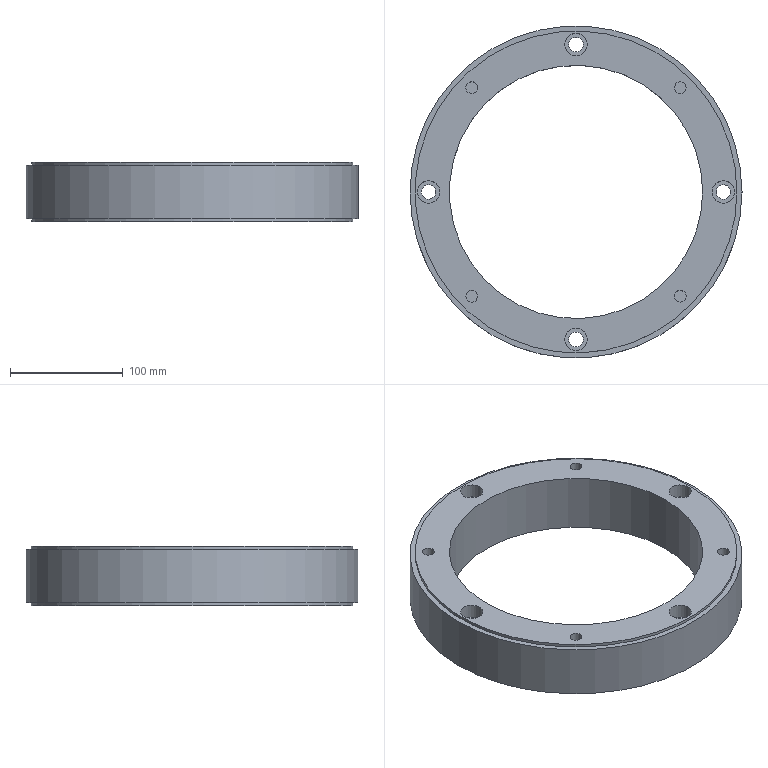CAM job | NX | 3-axis milling, drilling | part box 295 x 295 x 53 mm | stock box 301 x 301 x 54 mm
Tools:
number,name,description,diameter,corner_radius,flute_length,length,flutes
1,D63,Milling Tool-5 Parameters,63.0,0.0,50.0,75.0,2
7,D6A45,Milling Tool-5 Parameters,6.0,0.0,3.0,3.0,2
14,10.5ZT,Drilling Tool,10.5,0.0,35.0,50.0,2
13,13.0ZT,Drilling Tool,13.0,0.0,35.0,50.0,2
11,D10JING,Milling Tool-5 Parameters,10.0,0.0,50.0,75.0,2
17,D17R0.8,Milling Tool-5 Parameters,17.0,0.0,50.0,75.0,2
Operations:
program,operation,operation_type,tool,method,geometry_group,spindle_rpm,surface_speed,feed_per_tooth,feed_cut,feed_plunge,cut_length_mm,path_length_mm,cut_time_min,machine_time_min
1,FLOOR_WALL,VolumeBased25DMillingOperation,D63,METHOD,A,6500.0,1286.0,0.0962,1250.0,100.0,3469.547,3523.547,2.776,2.781
1,DRILLING,Operation,D6A45,METHOD,A,3000.0,56.0,0.0333,200.0,0.0,32.0,847.155,0.16,0.2415
1,DRILLING_COPY,Operation,10.5ZT,METHOD,A,1000.0,34.0,0.075,150.0,0.0,132.0,888.859,0.88,0.9557
1,DRILLING_COPY_COPY,Operation,13.0ZT,METHOD,A,1000.0,34.0,0.075,150.0,0.0,245.622,1116.103,1.637,1.724
1,HOLE_MILLING,CylinderMilling,D10JING,METHOD,A,6500.0,204.0,0.1269,1650.0,100.0,1885.815,2731.601,1.143,1.228
1,ADAPTIVE_MILLING,CavityMilling,D10JING,METHOD,A,6000.0,188.0,0.2917,3500.0,1000.0,2907.419,3021.419,0.8328,0.8442
1,ZLEVEL_PROFILE_COPY,ZLevelMilling,D17R0.8,METHOD,A,5000.0,267.0,0.25,2500.0,1000.0,47574.013,47688.013,19.062,19.073
1,ZLEVEL_PROFILE_1_COPY_1,ZLevelMilling,D6A45,METHOD,A,6500.0,122.0,0.0769,1000.0,100.0,384.678,2313.916,0.3847,0.5776
2,ZLEVEL_PROFILE,ZLevelMilling,D17R0.8,METHOD,A,5000.0,267.0,0.25,2500.0,1000.0,27688.08,27786.08,11.115,11.125